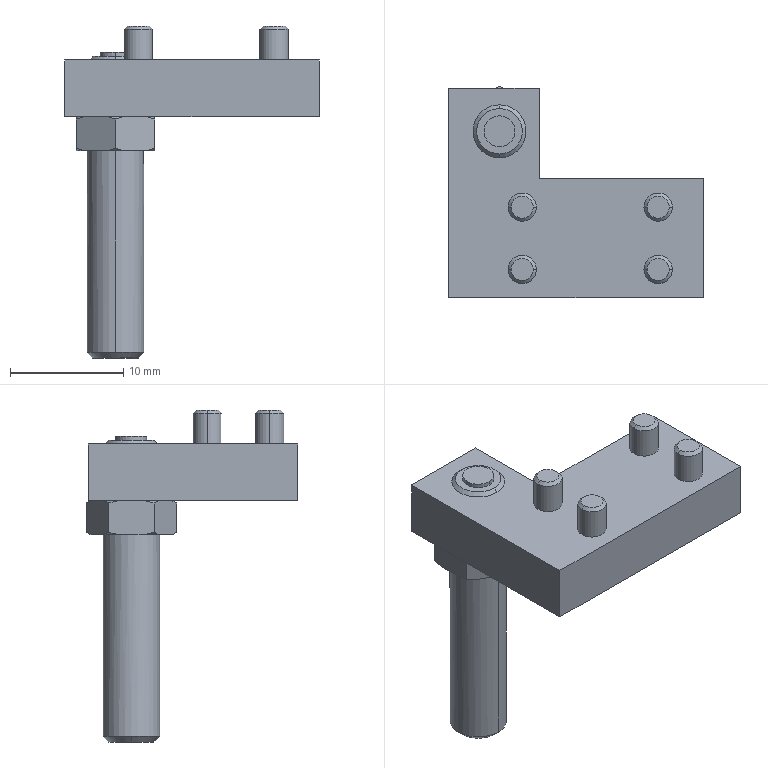Part | STEP file | QA-HI_MDX6_BB | 1 solid | 106 faces | box 22.5 x 18.7 x 29.3 mm | volume 2038 mm3 | plane 54 | cone 24 | cylinder 20 | spline 8 | commonest cylinder face diameters 2.5 x8 4.4 x8 2.744 x2 5 x2